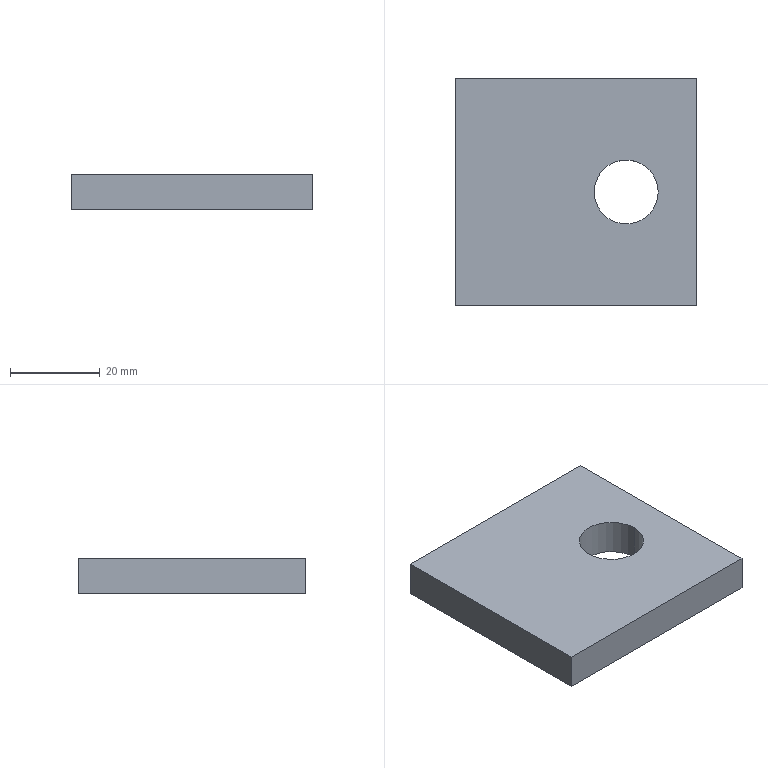Part | SolidWorks | features Extrusion 1 | 1 solid | 8 faces | box 53.848 x 50.8 x 8 mm | volume 20604 mm3 | plane 6 | cylinder 2 | commonest cylinder face diameters 14.275 x2
STEP:
#1=CARTESIAN_POINT('',(-7.137,0.,4.));
#2=VERTEX_POINT('',#1);
#3=CARTESIAN_POINT('',(7.137,0.,4.));
#4=VERTEX_POINT('',#3);
#5=CARTESIAN_POINT('',(0.,0.,4.));
#6=DIRECTION('',(0.,0.,1.));
#7=DIRECTION('',(1.,0.,0.));
#8=AXIS2_PLACEMENT_3D('',#5,#6,#7);
#9=CIRCLE('',#8,7.137);
#10=EDGE_CURVE('',#2,#4,#9,.T.);
#11=ORIENTED_EDGE('',*,*,#10,.T.);
#12=CARTESIAN_POINT('',(7.137,0.,-4.));
#13=VERTEX_POINT('',#12);
#14=CARTESIAN_POINT('',(7.137,0.,4.));
#15=DIRECTION('',(0.,0.,-1.));
#16=VECTOR('',#15,1000.);
#17=LINE('',#14,#16);
#18=EDGE_CURVE('',#4,#13,#17,.T.);
#19=ORIENTED_EDGE('',*,*,#18,.T.);
#20=CARTESIAN_POINT('',(-7.137,0.,-4.));
#21=VERTEX_POINT('',#20);
#22=CARTESIAN_POINT('',(0.,0.,-4.));
#23=DIRECTION('',(0.,0.,1.));
#24=DIRECTION('',(1.,0.,0.));
#25=AXIS2_PLACEMENT_3D('',#22,#23,#24);
#26=CIRCLE('',#25,7.137);
#27=EDGE_CURVE('',#21,#13,#26,.T.);
#28=ORIENTED_EDGE('',*,*,#27,.F.);
#29=CARTESIAN_POINT('',(-7.137,0.,4.));
#30=DIRECTION('',(0.,0.,-1.));
#31=VECTOR('',#30,1000.);
#32=LINE('',#29,#31);
#33=EDGE_CURVE('',#2,#21,#32,.T.);
#34=ORIENTED_EDGE('',*,*,#33,.F.);
#35=EDGE_LOOP('',(#11,#19,#28,#34));
#36=FACE_OUTER_BOUND('',#35,.T.);
#37=CARTESIAN_POINT('',(0.,0.,4.));
#38=DIRECTION('',(0.,0.,-1.));
#39=DIRECTION('',(-1.,0.,0.));
#40=AXIS2_PLACEMENT_3D('',#37,#38,#39);
#41=CYLINDRICAL_SURFACE('',#40,7.137);
#42=ADVANCED_FACE('',(#36),#41,.F.);
#43=CARTESIAN_POINT('',(-38.1,25.4,4.));
#44=VERTEX_POINT('',#43);
#45=CARTESIAN_POINT('',(-38.1,-25.4,4.));
#46=VERTEX_POINT('',#45);
#47=CARTESIAN_POINT('',(-38.1,25.4,4.));
#48=DIRECTION('',(0.,-1.,0.));
#49=VECTOR('',#48,1000.);
#50=LINE('',#47,#49);
#51=EDGE_CURVE('',#44,#46,#50,.T.);
#52=ORIENTED_EDGE('',*,*,#51,.T.);
#53=CARTESIAN_POINT('',(15.748,-25.4,4.));
#54=VERTEX_POINT('',#53);
#55=CARTESIAN_POINT('',(-38.1,-25.4,4.));
#56=DIRECTION('',(1.,0.,0.));
#57=VECTOR('',#56,1000.);
#58=LINE('',#55,#57);
#59=EDGE_CURVE('',#46,#54,#58,.T.);
#60=ORIENTED_EDGE('',*,*,#59,.T.);
#61=CARTESIAN_POINT('',(15.748,25.4,4.));
#62=VERTEX_POINT('',#61);
#63=CARTESIAN_POINT('',(15.748,25.4,4.));
#64=DIRECTION('',(0.,1.,0.));
#65=VECTOR('',#64,1000.);
#66=LINE('',#63,#65);
#67=EDGE_CURVE('',#54,#62,#66,.T.);
#68=ORIENTED_EDGE('',*,*,#67,.T.);
#69=CARTESIAN_POINT('',(-38.1,25.4,4.));
#70=DIRECTION('',(-1.,0.,0.));
#71=VECTOR('',#70,1000.);
#72=LINE('',#69,#71);
#73=EDGE_CURVE('',#62,#44,#72,.T.);
#74=ORIENTED_EDGE('',*,*,#73,.T.);
#75=EDGE_LOOP('',(#52,#60,#68,#74));
#76=FACE_OUTER_BOUND('',#75,.T.);
#77=ORIENTED_EDGE('',*,*,#10,.F.);
#78=CARTESIAN_POINT('',(0.,0.,4.));
#79=DIRECTION('',(0.,0.,1.));
#80=DIRECTION('',(1.,0.,0.));
#81=AXIS2_PLACEMENT_3D('',#78,#79,#80);
#82=CIRCLE('',#81,7.137);
#83=EDGE_CURVE('',#4,#2,#82,.T.);
#84=ORIENTED_EDGE('',*,*,#83,.F.);
#85=EDGE_LOOP('',(#77,#84));
#86=FACE_BOUND('',#85,.T.);
#87=CARTESIAN_POINT('',(0.,0.,4.));
#88=DIRECTION('',(0.,0.,1.));
#89=DIRECTION('',(1.,0.,0.));
#90=AXIS2_PLACEMENT_3D('',#87,#88,#89);
#91=PLANE('',#90);
#92=ADVANCED_FACE('',(#76,#86),#91,.T.);
#93=CARTESIAN_POINT('',(-38.1,25.4,-4.));
#94=VERTEX_POINT('',#93);
#95=CARTESIAN_POINT('',(-38.1,-25.4,-4.));
#96=VERTEX_POINT('',#95);
#97=CARTESIAN_POINT('',(-38.1,25.4,-4.));
#98=DIRECTION('',(0.,-1.,0.));
#99=VECTOR('',#98,1000.);
#100=LINE('',#97,#99);
#101=EDGE_CURVE('',#94,#96,#100,.T.);
#102=ORIENTED_EDGE('',*,*,#101,.F.);
#103=CARTESIAN_POINT('',(15.748,25.4,-4.));
#104=VERTEX_POINT('',#103);
#105=CARTESIAN_POINT('',(-38.1,25.4,-4.));
#106=DIRECTION('',(-1.,0.,0.));
#107=VECTOR('',#106,1000.);
#108=LINE('',#105,#107);
#109=EDGE_CURVE('',#104,#94,#108,.T.);
#110=ORIENTED_EDGE('',*,*,#109,.F.);
#111=CARTESIAN_POINT('',(15.748,-25.4,-4.));
#112=VERTEX_POINT('',#111);
#113=CARTESIAN_POINT('',(15.748,25.4,-4.));
#114=DIRECTION('',(0.,1.,0.));
#115=VECTOR('',#114,1000.);
#116=LINE('',#113,#115);
#117=EDGE_CURVE('',#112,#104,#116,.T.);
#118=ORIENTED_EDGE('',*,*,#117,.F.);
#119=CARTESIAN_POINT('',(-38.1,-25.4,-4.));
#120=DIRECTION('',(1.,0.,0.));
#121=VECTOR('',#120,1000.);
#122=LINE('',#119,#121);
#123=EDGE_CURVE('',#96,#112,#122,.T.);
#124=ORIENTED_EDGE('',*,*,#123,.F.);
#125=EDGE_LOOP('',(#102,#110,#118,#124));
#126=FACE_OUTER_BOUND('',#125,.T.);
#127=ORIENTED_EDGE('',*,*,#27,.T.);
#128=CARTESIAN_POINT('',(0.,0.,-4.));
#129=DIRECTION('',(0.,0.,1.));
#130=DIRECTION('',(1.,0.,0.));
#131=AXIS2_PLACEMENT_3D('',#128,#129,#130);
#132=CIRCLE('',#131,7.137);
#133=EDGE_CURVE('',#13,#21,#132,.T.);
#134=ORIENTED_EDGE('',*,*,#133,.T.);
#135=EDGE_LOOP('',(#127,#134));
#136=FACE_BOUND('',#135,.T.);
#137=CARTESIAN_POINT('',(0.,0.,-4.));
#138=DIRECTION('',(0.,0.,1.));
#139=DIRECTION('',(1.,0.,0.));
#140=AXIS2_PLACEMENT_3D('',#137,#138,#139);
#141=PLANE('',#140);
#142=ADVANCED_FACE('',(#126,#136),#141,.F.);
#143=ORIENTED_EDGE('',*,*,#101,.T.);
#144=CARTESIAN_POINT('',(-38.1,-25.4,4.));
#145=DIRECTION('',(0.,0.,-1.));
#146=VECTOR('',#145,1000.);
#147=LINE('',#144,#146);
#148=EDGE_CURVE('',#46,#96,#147,.T.);
#149=ORIENTED_EDGE('',*,*,#148,.F.);
#150=ORIENTED_EDGE('',*,*,#51,.F.);
#151=CARTESIAN_POINT('',(-38.1,25.4,4.));
#152=DIRECTION('',(0.,0.,-1.));
#153=VECTOR('',#152,1000.);
#154=LINE('',#151,#153);
#155=EDGE_CURVE('',#44,#94,#154,.T.);
#156=ORIENTED_EDGE('',*,*,#155,.T.);
#157=EDGE_LOOP('',(#143,#149,#150,#156));
#158=FACE_OUTER_BOUND('',#157,.T.);
#159=CARTESIAN_POINT('',(-38.1,25.4,4.));
#160=DIRECTION('',(1.,0.,0.));
#161=DIRECTION('',(0.,1.,0.));
#162=AXIS2_PLACEMENT_3D('',#159,#160,#161);
#163=PLANE('',#162);
#164=ADVANCED_FACE('',(#158),#163,.F.);
#165=ORIENTED_EDGE('',*,*,#123,.T.);
#166=CARTESIAN_POINT('',(15.748,-25.4,4.));
#167=DIRECTION('',(0.,0.,-1.));
#168=VECTOR('',#167,1000.);
#169=LINE('',#166,#168);
#170=EDGE_CURVE('',#54,#112,#169,.T.);
#171=ORIENTED_EDGE('',*,*,#170,.F.);
#172=ORIENTED_EDGE('',*,*,#59,.F.);
#173=ORIENTED_EDGE('',*,*,#148,.T.);
#174=EDGE_LOOP('',(#165,#171,#172,#173));
#175=FACE_OUTER_BOUND('',#174,.T.);
#176=CARTESIAN_POINT('',(-38.1,-25.4,4.));
#177=DIRECTION('',(0.,1.,0.));
#178=DIRECTION('',(0.,0.,1.));
#179=AXIS2_PLACEMENT_3D('',#176,#177,#178);
#180=PLANE('',#179);
#181=ADVANCED_FACE('',(#175),#180,.F.);
#182=ORIENTED_EDGE('',*,*,#117,.T.);
#183=CARTESIAN_POINT('',(15.748,25.4,4.));
#184=DIRECTION('',(0.,0.,-1.));
#185=VECTOR('',#184,1000.);
#186=LINE('',#183,#185);
#187=EDGE_CURVE('',#62,#104,#186,.T.);
#188=ORIENTED_EDGE('',*,*,#187,.F.);
#189=ORIENTED_EDGE('',*,*,#67,.F.);
#190=ORIENTED_EDGE('',*,*,#170,.T.);
#191=EDGE_LOOP('',(#182,#188,#189,#190));
#192=FACE_OUTER_BOUND('',#191,.T.);
#193=CARTESIAN_POINT('',(15.748,25.4,4.));
#194=DIRECTION('',(-1.,0.,0.));
#195=DIRECTION('',(0.,-1.,0.));
#196=AXIS2_PLACEMENT_3D('',#193,#194,#195);
#197=PLANE('',#196);
#198=ADVANCED_FACE('',(#192),#197,.F.);
#199=ORIENTED_EDGE('',*,*,#109,.T.);
#200=ORIENTED_EDGE('',*,*,#155,.F.);
#201=ORIENTED_EDGE('',*,*,#73,.F.);
#202=ORIENTED_EDGE('',*,*,#187,.T.);
#203=EDGE_LOOP('',(#199,#200,#201,#202));
#204=FACE_OUTER_BOUND('',#203,.T.);
#205=CARTESIAN_POINT('',(-38.1,25.4,4.));
#206=DIRECTION('',(0.,-1.,0.));
#207=DIRECTION('',(0.,0.,-1.));
#208=AXIS2_PLACEMENT_3D('',#205,#206,#207);
#209=PLANE('',#208);
#210=ADVANCED_FACE('',(#204),#209,.F.);
#211=ORIENTED_EDGE('',*,*,#18,.F.);
#212=ORIENTED_EDGE('',*,*,#83,.T.);
#213=ORIENTED_EDGE('',*,*,#33,.T.);
#214=ORIENTED_EDGE('',*,*,#133,.F.);
#215=EDGE_LOOP('',(#211,#212,#213,#214));
#216=FACE_OUTER_BOUND('',#215,.T.);
#217=CARTESIAN_POINT('',(0.,0.,4.));
#218=DIRECTION('',(0.,0.,-1.));
#219=DIRECTION('',(-1.,0.,0.));
#220=AXIS2_PLACEMENT_3D('',#217,#218,#219);
#221=CYLINDRICAL_SURFACE('',#220,7.137);
#222=ADVANCED_FACE('',(#216),#221,.F.);
#223=CLOSED_SHELL('',(#42,#92,#142,#164,#181,#198,#210,#222));
#224=MANIFOLD_SOLID_BREP('',#223);
#225=CARTESIAN_POINT('',(0.,0.,0.));
#226=DIRECTION('',(0.,0.,1.));
#227=DIRECTION('',(1.,0.,0.));
#228=AXIS2_PLACEMENT_3D('',#225,#226,#227);
#229=(LENGTH_UNIT()NAMED_UNIT(*)SI_UNIT(.MILLI.,.METRE.));
#230=UNCERTAINTY_MEASURE_WITH_UNIT(LENGTH_MEASURE(0.00001),#229,'','');
#231=(NAMED_UNIT(*)PLANE_ANGLE_UNIT()SI_UNIT($,.RADIAN.));
#232=(NAMED_UNIT(*)SI_UNIT($,.STERADIAN.)SOLID_ANGLE_UNIT());
#233=(GEOMETRIC_REPRESENTATION_CONTEXT(3)GLOBAL_UNCERTAINTY_ASSIGNED_CONTEXT((#230))GLOBAL_UNIT_ASSIGNED_CONTEXT((#229,#231,#232))REPRESENTATION_CONTEXT('',''));
#234=ADVANCED_BREP_SHAPE_REPRESENTATION('',(#224,#228),#233);